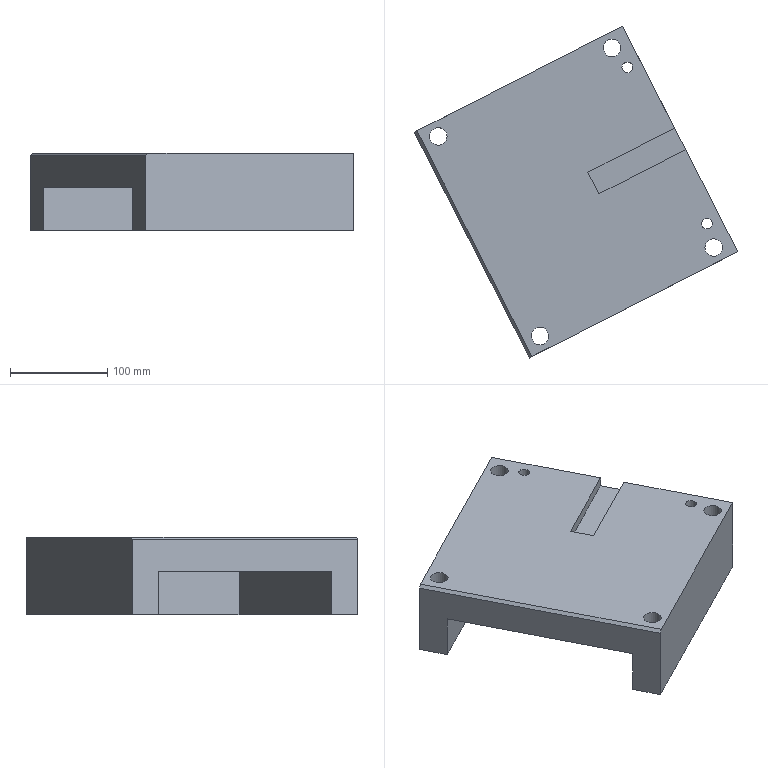Part | NX | features solid 2 | 1 solid | 29 faces | box 331.879 x 340.619 x 80 mm | volume 2957078 mm3 | plane 19 | cylinder 10 | commonest cylinder face diameters 18 x4 26 x4 11 x2
STEP:
#1=CARTESIAN_POINT('',(-1486.952,-451.806,260.));
#2=VERTEX_POINT('',#1);
#3=CARTESIAN_POINT('',(-1486.952,-451.806,250.));
#4=VERTEX_POINT('',#3);
#5=CARTESIAN_POINT('',(-1486.952,-451.806,270.));
#6=DIRECTION('',(0.,0.,-1.));
#7=VECTOR('',#6,1000.);
#8=LINE('',#5,#7);
#9=EDGE_CURVE('',#2,#4,#8,.T.);
#10=ORIENTED_EDGE('',*,*,#9,.F.);
#11=CARTESIAN_POINT('',(-1433.609,-556.499,260.));
#12=VERTEX_POINT('',#11);
#13=CARTESIAN_POINT('',(-1433.609,-556.499,260.));
#14=DIRECTION('',(-0.454,0.891,0.));
#15=VECTOR('',#14,1000.);
#16=LINE('',#13,#15);
#17=EDGE_CURVE('',#12,#2,#16,.T.);
#18=ORIENTED_EDGE('',*,*,#17,.F.);
#19=CARTESIAN_POINT('',(-1433.609,-556.499,180.));
#20=VERTEX_POINT('',#19);
#21=CARTESIAN_POINT('',(-1433.609,-556.499,260.));
#22=DIRECTION('',(0.,0.,-1.));
#23=VECTOR('',#22,1000.);
#24=LINE('',#21,#23);
#25=EDGE_CURVE('',#12,#20,#24,.T.);
#26=ORIENTED_EDGE('',*,*,#25,.T.);
#27=CARTESIAN_POINT('',(-1551.646,-324.838,180.));
#28=VERTEX_POINT('',#27);
#29=CARTESIAN_POINT('',(-1433.609,-556.499,180.));
#30=DIRECTION('',(-0.454,0.891,0.));
#31=VECTOR('',#30,1000.);
#32=LINE('',#29,#31);
#33=EDGE_CURVE('',#20,#28,#32,.T.);
#34=ORIENTED_EDGE('',*,*,#33,.T.);
#35=CARTESIAN_POINT('',(-1551.646,-324.838,260.));
#36=VERTEX_POINT('',#35);
#37=CARTESIAN_POINT('',(-1551.646,-324.838,260.));
#38=DIRECTION('',(0.,0.,-1.));
#39=VECTOR('',#38,1000.);
#40=LINE('',#37,#39);
#41=EDGE_CURVE('',#36,#28,#40,.T.);
#42=ORIENTED_EDGE('',*,*,#41,.F.);
#43=CARTESIAN_POINT('',(-1498.302,-429.531,260.));
#44=VERTEX_POINT('',#43);
#45=CARTESIAN_POINT('',(-1433.609,-556.499,260.));
#46=DIRECTION('',(-0.454,0.891,0.));
#47=VECTOR('',#46,1000.);
#48=LINE('',#45,#47);
#49=EDGE_CURVE('',#44,#36,#48,.T.);
#50=ORIENTED_EDGE('',*,*,#49,.F.);
#51=CARTESIAN_POINT('',(-1498.302,-429.531,250.));
#52=VERTEX_POINT('',#51);
#53=CARTESIAN_POINT('',(-1498.302,-429.531,250.));
#54=DIRECTION('',(0.,0.,1.));
#55=VECTOR('',#54,1000.);
#56=LINE('',#53,#55);
#57=EDGE_CURVE('',#52,#44,#56,.T.);
#58=ORIENTED_EDGE('',*,*,#57,.F.);
#59=CARTESIAN_POINT('',(-1486.952,-451.806,250.));
#60=DIRECTION('',(-0.454,0.891,0.));
#61=VECTOR('',#60,1000.);
#62=LINE('',#59,#61);
#63=EDGE_CURVE('',#4,#52,#62,.T.);
#64=ORIENTED_EDGE('',*,*,#63,.F.);
#65=EDGE_LOOP('',(#10,#18,#26,#34,#42,#50,#58,#64));
#66=FACE_BOUND('',#65,.T.);
#67=CARTESIAN_POINT('',(-1433.609,-556.499,260.));
#68=DIRECTION('',(-0.891,-0.454,0.));
#69=DIRECTION('',(0.,0.,1.));
#70=AXIS2_PLACEMENT_3D('',#67,#68,#69);
#71=PLANE('',#70);
#72=ADVANCED_FACE('',(#66),#71,.F.);
#73=CARTESIAN_POINT('',(-1628.42,-638.926,260.));
#74=VERTEX_POINT('',#73);
#75=CARTESIAN_POINT('',(-1636.44,-643.012,260.));
#76=DIRECTION('',(0.,0.,-1.));
#77=DIRECTION('',(0.891,0.454,0.));
#78=AXIS2_PLACEMENT_3D('',#75,#76,#77);
#79=CIRCLE('',#78,9.);
#80=EDGE_CURVE('',#74,#74,#79,.T.);
#81=ORIENTED_EDGE('',*,*,#80,.T.);
#82=EDGE_LOOP('',(#81));
#83=FACE_BOUND('',#82,.T.);
#84=CARTESIAN_POINT('',(-1450.219,-548.128,260.));
#85=VERTEX_POINT('',#84);
#86=CARTESIAN_POINT('',(-1458.238,-552.214,260.));
#87=DIRECTION('',(0.,0.,-1.));
#88=DIRECTION('',(0.891,0.454,0.));
#89=AXIS2_PLACEMENT_3D('',#86,#87,#88);
#90=CIRCLE('',#89,9.);
#91=EDGE_CURVE('',#85,#85,#90,.T.);
#92=ORIENTED_EDGE('',*,*,#91,.T.);
#93=EDGE_LOOP('',(#92));
#94=FACE_BOUND('',#93,.T.);
#95=CARTESIAN_POINT('',(-1460.232,-525.172,260.));
#96=VERTEX_POINT('',#95);
#97=CARTESIAN_POINT('',(-1465.133,-527.669,260.));
#98=DIRECTION('',(0.,0.,-1.));
#99=DIRECTION('',(0.891,0.454,0.));
#100=AXIS2_PLACEMENT_3D('',#97,#98,#99);
#101=CIRCLE('',#100,5.5);
#102=EDGE_CURVE('',#96,#96,#101,.T.);
#103=ORIENTED_EDGE('',*,*,#102,.T.);
#104=EDGE_LOOP('',(#103));
#105=FACE_BOUND('',#104,.T.);
#106=CARTESIAN_POINT('',(-1541.951,-364.791,260.));
#107=VERTEX_POINT('',#106);
#108=CARTESIAN_POINT('',(-1546.851,-367.288,260.));
#109=DIRECTION('',(0.,0.,-1.));
#110=DIRECTION('',(0.891,0.454,0.));
#111=AXIS2_PLACEMENT_3D('',#108,#109,#110);
#112=CIRCLE('',#111,5.5);
#113=EDGE_CURVE('',#107,#107,#112,.T.);
#114=ORIENTED_EDGE('',*,*,#113,.T.);
#115=EDGE_LOOP('',(#114));
#116=FACE_BOUND('',#115,.T.);
#117=CARTESIAN_POINT('',(-1554.637,-343.197,260.));
#118=VERTEX_POINT('',#117);
#119=CARTESIAN_POINT('',(-1562.656,-347.283,260.));
#120=DIRECTION('',(0.,0.,-1.));
#121=DIRECTION('',(0.891,0.454,0.));
#122=AXIS2_PLACEMENT_3D('',#119,#120,#121);
#123=CIRCLE('',#122,9.);
#124=EDGE_CURVE('',#118,#118,#123,.T.);
#125=ORIENTED_EDGE('',*,*,#124,.T.);
#126=EDGE_LOOP('',(#125));
#127=FACE_BOUND('',#126,.T.);
#128=CARTESIAN_POINT('',(-1732.838,-433.995,260.));
#129=VERTEX_POINT('',#128);
#130=CARTESIAN_POINT('',(-1740.857,-438.081,260.));
#131=DIRECTION('',(0.,0.,-1.));
#132=DIRECTION('',(0.891,0.454,0.));
#133=AXIS2_PLACEMENT_3D('',#130,#131,#132);
#134=CIRCLE('',#133,9.);
#135=EDGE_CURVE('',#129,#129,#134,.T.);
#136=ORIENTED_EDGE('',*,*,#135,.T.);
#137=EDGE_LOOP('',(#136));
#138=FACE_BOUND('',#137,.T.);
#139=CARTESIAN_POINT('',(-1576.053,-497.205,260.));
#140=VERTEX_POINT('',#139);
#141=CARTESIAN_POINT('',(-1587.403,-474.93,260.));
#142=VERTEX_POINT('',#141);
#143=CARTESIAN_POINT('',(-1522.709,-601.899,260.));
#144=DIRECTION('',(-0.454,0.891,0.));
#145=VECTOR('',#144,1000.);
#146=LINE('',#143,#145);
#147=EDGE_CURVE('',#140,#142,#146,.T.);
#148=ORIENTED_EDGE('',*,*,#147,.T.);
#149=CARTESIAN_POINT('',(-1498.302,-429.531,260.));
#150=DIRECTION('',(-0.891,-0.454,0.));
#151=VECTOR('',#150,1000.);
#152=LINE('',#149,#151);
#153=EDGE_CURVE('',#44,#142,#152,.T.);
#154=ORIENTED_EDGE('',*,*,#153,.F.);
#155=ORIENTED_EDGE('',*,*,#49,.T.);
#156=CARTESIAN_POINT('',(-1762.815,-432.434,260.));
#157=VERTEX_POINT('',#156);
#158=CARTESIAN_POINT('',(-1551.646,-324.838,260.));
#159=DIRECTION('',(-0.891,-0.454,0.));
#160=VECTOR('',#159,1000.);
#161=LINE('',#158,#160);
#162=EDGE_CURVE('',#36,#157,#161,.T.);
#163=ORIENTED_EDGE('',*,*,#162,.T.);
#164=CARTESIAN_POINT('',(-1644.777,-664.095,260.));
#165=VERTEX_POINT('',#164);
#166=CARTESIAN_POINT('',(-1644.777,-664.095,260.));
#167=DIRECTION('',(-0.454,0.891,0.));
#168=VECTOR('',#167,1000.);
#169=LINE('',#166,#168);
#170=EDGE_CURVE('',#165,#157,#169,.T.);
#171=ORIENTED_EDGE('',*,*,#170,.F.);
#172=CARTESIAN_POINT('',(-1433.609,-556.499,260.));
#173=DIRECTION('',(-0.891,-0.454,0.));
#174=VECTOR('',#173,1000.);
#175=LINE('',#172,#174);
#176=EDGE_CURVE('',#12,#165,#175,.T.);
#177=ORIENTED_EDGE('',*,*,#176,.F.);
#178=ORIENTED_EDGE('',*,*,#17,.T.);
#179=CARTESIAN_POINT('',(-1486.952,-451.806,260.));
#180=DIRECTION('',(0.891,0.454,0.));
#181=VECTOR('',#180,1000.);
#182=LINE('',#179,#181);
#183=EDGE_CURVE('',#140,#2,#182,.T.);
#184=ORIENTED_EDGE('',*,*,#183,.F.);
#185=EDGE_LOOP('',(#148,#154,#155,#163,#171,#177,#178,#184));
#186=FACE_BOUND('',#185,.T.);
#187=CARTESIAN_POINT('',(-1433.609,-556.499,260.));
#188=DIRECTION('',(0.,0.,1.));
#189=DIRECTION('',(0.891,0.454,0.));
#190=AXIS2_PLACEMENT_3D('',#187,#188,#189);
#191=PLANE('',#190);
#192=ADVANCED_FACE('',(#83,#94,#105,#116,#127,#138,#186),#191,.T.);
#193=CARTESIAN_POINT('',(-1647.45,-665.457,257.));
#194=VERTEX_POINT('',#193);
#195=CARTESIAN_POINT('',(-1765.488,-433.795,257.));
#196=VERTEX_POINT('',#195);
#197=CARTESIAN_POINT('',(-1647.45,-665.457,257.));
#198=DIRECTION('',(-0.454,0.891,0.));
#199=VECTOR('',#198,1000.);
#200=LINE('',#197,#199);
#201=EDGE_CURVE('',#194,#196,#200,.T.);
#202=ORIENTED_EDGE('',*,*,#201,.F.);
#203=CARTESIAN_POINT('',(-1644.777,-664.095,260.));
#204=DIRECTION('',(-0.63,-0.321,-0.7071));
#205=VECTOR('',#204,1000.);
#206=LINE('',#203,#205);
#207=EDGE_CURVE('',#165,#194,#206,.T.);
#208=ORIENTED_EDGE('',*,*,#207,.F.);
#209=ORIENTED_EDGE('',*,*,#170,.T.);
#210=CARTESIAN_POINT('',(-1762.815,-432.434,260.));
#211=DIRECTION('',(-0.63,-0.321,-0.7071));
#212=VECTOR('',#211,1000.);
#213=LINE('',#210,#212);
#214=EDGE_CURVE('',#157,#196,#213,.T.);
#215=ORIENTED_EDGE('',*,*,#214,.T.);
#216=EDGE_LOOP('',(#202,#208,#209,#215));
#217=FACE_BOUND('',#216,.T.);
#218=CARTESIAN_POINT('',(-1644.777,-664.095,260.));
#219=DIRECTION('',(-0.63,-0.321,0.7071));
#220=DIRECTION('',(0.63,0.321,0.7071));
#221=AXIS2_PLACEMENT_3D('',#218,#219,#220);
#222=PLANE('',#221);
#223=ADVANCED_FACE('',(#217),#222,.T.);
#224=CARTESIAN_POINT('',(-1661.07,-638.727,225.));
#225=VERTEX_POINT('',#224);
#226=CARTESIAN_POINT('',(-1661.07,-638.727,180.));
#227=VERTEX_POINT('',#226);
#228=CARTESIAN_POINT('',(-1661.07,-638.727,185.));
#229=DIRECTION('',(0.,0.,-1.));
#230=VECTOR('',#229,1000.);
#231=LINE('',#228,#230);
#232=EDGE_CURVE('',#225,#227,#231,.T.);
#233=ORIENTED_EDGE('',*,*,#232,.T.);
#234=CARTESIAN_POINT('',(-1647.45,-665.457,180.));
#235=VERTEX_POINT('',#234);
#236=CARTESIAN_POINT('',(-1647.45,-665.457,180.));
#237=DIRECTION('',(-0.454,0.891,0.));
#238=VECTOR('',#237,1000.);
#239=LINE('',#236,#238);
#240=EDGE_CURVE('',#227,#235,#239,.F.);
#241=ORIENTED_EDGE('',*,*,#240,.T.);
#242=CARTESIAN_POINT('',(-1647.45,-665.457,185.));
#243=DIRECTION('',(0.,0.,-1.));
#244=VECTOR('',#243,1000.);
#245=LINE('',#242,#244);
#246=EDGE_CURVE('',#194,#235,#245,.T.);
#247=ORIENTED_EDGE('',*,*,#246,.F.);
#248=ORIENTED_EDGE('',*,*,#201,.T.);
#249=CARTESIAN_POINT('',(-1765.488,-433.795,180.));
#250=VERTEX_POINT('',#249);
#251=CARTESIAN_POINT('',(-1765.488,-433.795,250.));
#252=DIRECTION('',(0.,0.,-1.));
#253=VECTOR('',#252,1000.);
#254=LINE('',#251,#253);
#255=EDGE_CURVE('',#196,#250,#254,.T.);
#256=ORIENTED_EDGE('',*,*,#255,.T.);
#257=CARTESIAN_POINT('',(-1751.868,-460.526,180.));
#258=VERTEX_POINT('',#257);
#259=CARTESIAN_POINT('',(-1765.488,-433.795,180.));
#260=DIRECTION('',(0.454,-0.891,0.));
#261=VECTOR('',#260,1000.);
#262=LINE('',#259,#261);
#263=EDGE_CURVE('',#250,#258,#262,.T.);
#264=ORIENTED_EDGE('',*,*,#263,.T.);
#265=CARTESIAN_POINT('',(-1751.868,-460.526,225.));
#266=VERTEX_POINT('',#265);
#267=CARTESIAN_POINT('',(-1751.868,-460.526,250.));
#268=DIRECTION('',(0.,0.,-1.));
#269=VECTOR('',#268,1000.);
#270=LINE('',#267,#269);
#271=EDGE_CURVE('',#266,#258,#270,.T.);
#272=ORIENTED_EDGE('',*,*,#271,.F.);
#273=CARTESIAN_POINT('',(-1661.07,-638.727,225.));
#274=DIRECTION('',(-0.454,0.891,0.));
#275=VECTOR('',#274,1000.);
#276=LINE('',#273,#275);
#277=EDGE_CURVE('',#225,#266,#276,.T.);
#278=ORIENTED_EDGE('',*,*,#277,.F.);
#279=EDGE_LOOP('',(#233,#241,#247,#248,#256,#264,#272,#278));
#280=FACE_BOUND('',#279,.T.);
#281=CARTESIAN_POINT('',(-1647.45,-665.457,185.));
#282=DIRECTION('',(-0.891,-0.454,0.));
#283=DIRECTION('',(0.,0.,1.));
#284=AXIS2_PLACEMENT_3D('',#281,#282,#283);
#285=PLANE('',#284);
#286=ADVANCED_FACE('',(#280),#285,.T.);
#287=CARTESIAN_POINT('',(-1541.951,-364.791,180.));
#288=VERTEX_POINT('',#287);
#289=CARTESIAN_POINT('',(-1546.851,-367.288,180.));
#290=DIRECTION('',(0.,0.,-1.));
#291=DIRECTION('',(0.891,0.454,0.));
#292=AXIS2_PLACEMENT_3D('',#289,#290,#291);
#293=CIRCLE('',#292,5.5);
#294=EDGE_CURVE('',#288,#288,#293,.T.);
#295=ORIENTED_EDGE('',*,*,#294,.F.);
#296=EDGE_LOOP('',(#295));
#297=FACE_BOUND('',#296,.T.);
#298=CARTESIAN_POINT('',(-1460.232,-525.172,180.));
#299=VERTEX_POINT('',#298);
#300=CARTESIAN_POINT('',(-1465.133,-527.669,180.));
#301=DIRECTION('',(0.,0.,-1.));
#302=DIRECTION('',(0.891,0.454,0.));
#303=AXIS2_PLACEMENT_3D('',#300,#301,#302);
#304=CIRCLE('',#303,5.5);
#305=EDGE_CURVE('',#299,#299,#304,.T.);
#306=ORIENTED_EDGE('',*,*,#305,.F.);
#307=EDGE_LOOP('',(#306));
#308=FACE_BOUND('',#307,.T.);
#309=CARTESIAN_POINT('',(-1729.274,-432.179,180.));
#310=VERTEX_POINT('',#309);
#311=CARTESIAN_POINT('',(-1740.857,-438.081,180.));
#312=DIRECTION('',(0.,0.,-1.));
#313=DIRECTION('',(0.891,0.454,0.));
#314=AXIS2_PLACEMENT_3D('',#311,#312,#313);
#315=CIRCLE('',#314,13.);
#316=EDGE_CURVE('',#310,#310,#315,.T.);
#317=ORIENTED_EDGE('',*,*,#316,.F.);
#318=EDGE_LOOP('',(#317));
#319=FACE_BOUND('',#318,.T.);
#320=CARTESIAN_POINT('',(-1551.073,-341.381,180.));
#321=VERTEX_POINT('',#320);
#322=CARTESIAN_POINT('',(-1562.656,-347.283,180.));
#323=DIRECTION('',(0.,0.,-1.));
#324=DIRECTION('',(0.891,0.454,0.));
#325=AXIS2_PLACEMENT_3D('',#322,#323,#324);
#326=CIRCLE('',#325,13.);
#327=EDGE_CURVE('',#321,#321,#326,.T.);
#328=ORIENTED_EDGE('',*,*,#327,.F.);
#329=EDGE_LOOP('',(#328));
#330=FACE_BOUND('',#329,.T.);
#331=CARTESIAN_POINT('',(-1624.856,-637.11,180.));
#332=VERTEX_POINT('',#331);
#333=CARTESIAN_POINT('',(-1636.44,-643.012,180.));
#334=DIRECTION('',(0.,0.,-1.));
#335=DIRECTION('',(0.891,0.454,0.));
#336=AXIS2_PLACEMENT_3D('',#333,#334,#335);
#337=CIRCLE('',#336,13.);
#338=EDGE_CURVE('',#332,#332,#337,.T.);
#339=ORIENTED_EDGE('',*,*,#338,.F.);
#340=EDGE_LOOP('',(#339));
#341=FACE_BOUND('',#340,.T.);
#342=CARTESIAN_POINT('',(-1446.655,-546.312,180.));
#343=VERTEX_POINT('',#342);
#344=CARTESIAN_POINT('',(-1458.238,-552.214,180.));
#345=DIRECTION('',(0.,0.,-1.));
#346=DIRECTION('',(0.891,0.454,0.));
#347=AXIS2_PLACEMENT_3D('',#344,#345,#346);
#348=CIRCLE('',#347,13.);
#349=EDGE_CURVE('',#343,#343,#348,.T.);
#350=ORIENTED_EDGE('',*,*,#349,.F.);
#351=EDGE_LOOP('',(#350));
#352=FACE_BOUND('',#351,.T.);
#353=ORIENTED_EDGE('',*,*,#33,.F.);
#354=CARTESIAN_POINT('',(-1433.609,-556.499,180.));
#355=DIRECTION('',(-0.891,-0.454,0.));
#356=VECTOR('',#355,1000.);
#357=LINE('',#354,#356);
#358=EDGE_CURVE('',#20,#235,#357,.T.);
#359=ORIENTED_EDGE('',*,*,#358,.T.);
#360=ORIENTED_EDGE('',*,*,#240,.F.);
#361=CARTESIAN_POINT('',(-1473.958,-543.389,180.));
#362=VERTEX_POINT('',#361);
#363=CARTESIAN_POINT('',(-1447.228,-529.769,180.));
#364=DIRECTION('',(-0.891,-0.454,0.));
#365=VECTOR('',#364,1000.);
#366=LINE('',#363,#365);
#367=EDGE_CURVE('',#362,#227,#366,.T.);
#368=ORIENTED_EDGE('',*,*,#367,.F.);
#369=CARTESIAN_POINT('',(-1564.757,-365.188,180.));
#370=VERTEX_POINT('',#369);
#371=CARTESIAN_POINT('',(-1473.958,-543.389,180.));
#372=DIRECTION('',(-0.454,0.891,0.));
#373=VECTOR('',#372,1000.);
#374=LINE('',#371,#373);
#375=EDGE_CURVE('',#362,#370,#374,.T.);
#376=ORIENTED_EDGE('',*,*,#375,.T.);
#377=CARTESIAN_POINT('',(-1538.026,-351.568,180.));
#378=DIRECTION('',(-0.891,-0.454,0.));
#379=VECTOR('',#378,1000.);
#380=LINE('',#377,#379);
#381=EDGE_CURVE('',#370,#258,#380,.T.);
#382=ORIENTED_EDGE('',*,*,#381,.T.);
#383=ORIENTED_EDGE('',*,*,#263,.F.);
#384=CARTESIAN_POINT('',(-1551.646,-324.838,180.));
#385=DIRECTION('',(-0.891,-0.454,0.));
#386=VECTOR('',#385,1000.);
#387=LINE('',#384,#386);
#388=EDGE_CURVE('',#28,#250,#387,.T.);
#389=ORIENTED_EDGE('',*,*,#388,.F.);
#390=EDGE_LOOP('',(#353,#359,#360,#368,#376,#382,#383,#389));
#391=FACE_BOUND('',#390,.T.);
#392=CARTESIAN_POINT('',(-1433.609,-556.499,180.));
#393=DIRECTION('',(0.,0.,1.));
#394=DIRECTION('',(0.891,0.454,0.));
#395=AXIS2_PLACEMENT_3D('',#392,#393,#394);
#396=PLANE('',#395);
#397=ADVANCED_FACE('',(#297,#308,#319,#330,#341,#352,#391),#396,.F.);
#398=ORIENTED_EDGE('',*,*,#207,.T.);
#399=ORIENTED_EDGE('',*,*,#246,.T.);
#400=ORIENTED_EDGE('',*,*,#358,.F.);
#401=ORIENTED_EDGE('',*,*,#25,.F.);
#402=ORIENTED_EDGE('',*,*,#176,.T.);
#403=EDGE_LOOP('',(#398,#399,#400,#401,#402));
#404=FACE_BOUND('',#403,.T.);
#405=CARTESIAN_POINT('',(-1647.45,-665.457,257.));
#406=DIRECTION('',(-0.454,0.891,0.));
#407=DIRECTION('',(0.,0.,-1.));
#408=AXIS2_PLACEMENT_3D('',#405,#406,#407);
#409=PLANE('',#408);
#410=ADVANCED_FACE('',(#404),#409,.F.);
#411=CARTESIAN_POINT('',(-1473.958,-543.389,225.));
#412=VERTEX_POINT('',#411);
#413=CARTESIAN_POINT('',(-1473.958,-543.389,225.));
#414=DIRECTION('',(0.,0.,-1.));
#415=VECTOR('',#414,1000.);
#416=LINE('',#413,#415);
#417=EDGE_CURVE('',#412,#362,#416,.T.);
#418=ORIENTED_EDGE('',*,*,#417,.T.);
#419=ORIENTED_EDGE('',*,*,#367,.T.);
#420=ORIENTED_EDGE('',*,*,#232,.F.);
#421=CARTESIAN_POINT('',(-1487.324,-550.199,225.));
#422=DIRECTION('',(0.891,0.454,0.));
#423=VECTOR('',#422,1000.);
#424=LINE('',#421,#423);
#425=EDGE_CURVE('',#225,#412,#424,.T.);
#426=ORIENTED_EDGE('',*,*,#425,.T.);
#427=EDGE_LOOP('',(#418,#419,#420,#426));
#428=FACE_BOUND('',#427,.T.);
#429=CARTESIAN_POINT('',(-1661.07,-638.727,257.));
#430=DIRECTION('',(-0.454,0.891,0.));
#431=DIRECTION('',(0.,0.,-1.));
#432=AXIS2_PLACEMENT_3D('',#429,#430,#431);
#433=PLANE('',#432);
#434=ADVANCED_FACE('',(#428),#433,.T.);
#435=CARTESIAN_POINT('',(-1564.757,-365.188,225.));
#436=VERTEX_POINT('',#435);
#437=CARTESIAN_POINT('',(-1578.122,-371.998,225.));
#438=DIRECTION('',(0.891,0.454,0.));
#439=VECTOR('',#438,1000.);
#440=LINE('',#437,#439);
#441=EDGE_CURVE('',#266,#436,#440,.T.);
#442=ORIENTED_EDGE('',*,*,#441,.T.);
#443=CARTESIAN_POINT('',(-1473.958,-543.389,225.));
#444=DIRECTION('',(-0.454,0.891,0.));
#445=VECTOR('',#444,1000.);
#446=LINE('',#443,#445);
#447=EDGE_CURVE('',#412,#436,#446,.T.);
#448=ORIENTED_EDGE('',*,*,#447,.F.);
#449=ORIENTED_EDGE('',*,*,#425,.F.);
#450=ORIENTED_EDGE('',*,*,#277,.T.);
#451=EDGE_LOOP('',(#442,#448,#449,#450));
#452=FACE_BOUND('',#451,.T.);
#453=CARTESIAN_POINT('',(-1487.324,-550.199,225.));
#454=DIRECTION('',(0.,0.,-1.));
#455=DIRECTION('',(-0.891,-0.454,0.));
#456=AXIS2_PLACEMENT_3D('',#453,#454,#455);
#457=PLANE('',#456);
#458=ADVANCED_FACE('',(#452),#457,.T.);
#459=CARTESIAN_POINT('',(-1564.757,-365.188,225.));
#460=DIRECTION('',(0.,0.,-1.));
#461=VECTOR('',#460,1000.);
#462=LINE('',#459,#461);
#463=EDGE_CURVE('',#436,#370,#462,.T.);
#464=ORIENTED_EDGE('',*,*,#463,.T.);
#465=ORIENTED_EDGE('',*,*,#375,.F.);
#466=ORIENTED_EDGE('',*,*,#417,.F.);
#467=ORIENTED_EDGE('',*,*,#447,.T.);
#468=EDGE_LOOP('',(#464,#465,#466,#467));
#469=FACE_BOUND('',#468,.T.);
#470=CARTESIAN_POINT('',(-1473.958,-543.389,225.));
#471=DIRECTION('',(-0.891,-0.454,0.));
#472=DIRECTION('',(0.,0.,1.));
#473=AXIS2_PLACEMENT_3D('',#470,#471,#472);
#474=PLANE('',#473);
#475=ADVANCED_FACE('',(#469),#474,.T.);
#476=ORIENTED_EDGE('',*,*,#255,.F.);
#477=ORIENTED_EDGE('',*,*,#214,.F.);
#478=ORIENTED_EDGE('',*,*,#162,.F.);
#479=ORIENTED_EDGE('',*,*,#41,.T.);
#480=ORIENTED_EDGE('',*,*,#388,.T.);
#481=EDGE_LOOP('',(#476,#477,#478,#479,#480));
#482=FACE_BOUND('',#481,.T.);
#483=CARTESIAN_POINT('',(-1765.488,-433.795,180.));
#484=DIRECTION('',(0.454,-0.891,0.));
#485=DIRECTION('',(0.,0.,1.));
#486=AXIS2_PLACEMENT_3D('',#483,#484,#485);
#487=PLANE('',#486);
#488=ADVANCED_FACE('',(#482),#487,.F.);
#489=ORIENTED_EDGE('',*,*,#271,.T.);
#490=ORIENTED_EDGE('',*,*,#381,.F.);
#491=ORIENTED_EDGE('',*,*,#463,.F.);
#492=ORIENTED_EDGE('',*,*,#441,.F.);
#493=EDGE_LOOP('',(#489,#490,#491,#492));
#494=FACE_BOUND('',#493,.T.);
#495=CARTESIAN_POINT('',(-1751.868,-460.526,180.));
#496=DIRECTION('',(0.454,-0.891,0.));
#497=DIRECTION('',(0.,0.,1.));
#498=AXIS2_PLACEMENT_3D('',#495,#496,#497);
#499=PLANE('',#498);
#500=ADVANCED_FACE('',(#494),#499,.T.);
#501=CARTESIAN_POINT('',(-1446.655,-546.312,200.));
#502=VERTEX_POINT('',#501);
#503=CARTESIAN_POINT('',(-1458.238,-552.214,200.));
#504=DIRECTION('',(0.,0.,-1.));
#505=DIRECTION('',(0.891,0.454,0.));
#506=AXIS2_PLACEMENT_3D('',#503,#504,#505);
#507=CIRCLE('',#506,13.);
#508=EDGE_CURVE('',#502,#502,#507,.T.);
#509=ORIENTED_EDGE('',*,*,#508,.F.);
#510=EDGE_LOOP('',(#509));
#511=FACE_BOUND('',#510,.T.);
#512=ORIENTED_EDGE('',*,*,#349,.T.);
#513=EDGE_LOOP('',(#512));
#514=FACE_BOUND('',#513,.T.);
#515=CARTESIAN_POINT('',(-1458.238,-552.214,169.));
#516=DIRECTION('',(0.,0.,1.));
#517=DIRECTION('',(0.891,0.454,0.));
#518=AXIS2_PLACEMENT_3D('',#515,#516,#517);
#519=CYLINDRICAL_SURFACE('',#518,13.);
#520=ADVANCED_FACE('',(#511,#514),#519,.F.);
#521=CARTESIAN_POINT('',(-1450.219,-548.128,200.));
#522=VERTEX_POINT('',#521);
#523=CARTESIAN_POINT('',(-1458.238,-552.214,200.));
#524=DIRECTION('',(0.,0.,-1.));
#525=DIRECTION('',(0.891,0.454,0.));
#526=AXIS2_PLACEMENT_3D('',#523,#524,#525);
#527=CIRCLE('',#526,9.);
#528=EDGE_CURVE('',#522,#522,#527,.T.);
#529=ORIENTED_EDGE('',*,*,#528,.F.);
#530=EDGE_LOOP('',(#529));
#531=FACE_BOUND('',#530,.T.);
#532=ORIENTED_EDGE('',*,*,#508,.T.);
#533=EDGE_LOOP('',(#532));
#534=FACE_BOUND('',#533,.T.);
#535=CARTESIAN_POINT('',(-1458.238,-552.214,200.));
#536=DIRECTION('',(0.,0.,1.));
#537=DIRECTION('',(0.891,0.454,0.));
#538=AXIS2_PLACEMENT_3D('',#535,#536,#537);
#539=PLANE('',#538);
#540=ADVANCED_FACE('',(#531,#534),#539,.F.);
#541=CARTESIAN_POINT('',(-1624.856,-637.11,200.));
#542=VERTEX_POINT('',#541);
#543=CARTESIAN_POINT('',(-1636.44,-643.012,200.));
#544=DIRECTION('',(0.,0.,-1.));
#545=DIRECTION('',(0.891,0.454,0.));
#546=AXIS2_PLACEMENT_3D('',#543,#544,#545);
#547=CIRCLE('',#546,13.);
#548=EDGE_CURVE('',#542,#542,#547,.T.);
#549=ORIENTED_EDGE('',*,*,#548,.F.);
#550=EDGE_LOOP('',(#549));
#551=FACE_BOUND('',#550,.T.);
#552=ORIENTED_EDGE('',*,*,#338,.T.);
#553=EDGE_LOOP('',(#552));
#554=FACE_BOUND('',#553,.T.);
#555=CARTESIAN_POINT('',(-1636.44,-643.012,169.));
#556=DIRECTION('',(0.,0.,1.));
#557=DIRECTION('',(0.891,0.454,0.));
#558=AXIS2_PLACEMENT_3D('',#555,#556,#557);
#559=CYLINDRICAL_SURFACE('',#558,13.);
#560=ADVANCED_FACE('',(#551,#554),#559,.F.);
#561=CARTESIAN_POINT('',(-1628.42,-638.926,200.));
#562=VERTEX_POINT('',#561);
#563=CARTESIAN_POINT('',(-1636.44,-643.012,200.));
#564=DIRECTION('',(0.,0.,-1.));
#565=DIRECTION('',(0.891,0.454,0.));
#566=AXIS2_PLACEMENT_3D('',#563,#564,#565);
#567=CIRCLE('',#566,9.);
#568=EDGE_CURVE('',#562,#562,#567,.T.);
#569=ORIENTED_EDGE('',*,*,#568,.F.);
#570=EDGE_LOOP('',(#569));
#571=FACE_BOUND('',#570,.T.);
#572=ORIENTED_EDGE('',*,*,#548,.T.);
#573=EDGE_LOOP('',(#572));
#574=FACE_BOUND('',#573,.T.);
#575=CARTESIAN_POINT('',(-1636.44,-643.012,200.));
#576=DIRECTION('',(0.,0.,1.));
#577=DIRECTION('',(0.891,0.454,0.));
#578=AXIS2_PLACEMENT_3D('',#575,#576,#577);
#579=PLANE('',#578);
#580=ADVANCED_FACE('',(#571,#574),#579,.F.);
#581=CARTESIAN_POINT('',(-1551.073,-341.381,200.));
#582=VERTEX_POINT('',#581);
#583=CARTESIAN_POINT('',(-1562.656,-347.283,200.));
#584=DIRECTION('',(0.,0.,-1.));
#585=DIRECTION('',(0.891,0.454,0.));
#586=AXIS2_PLACEMENT_3D('',#583,#584,#585);
#587=CIRCLE('',#586,13.);
#588=EDGE_CURVE('',#582,#582,#587,.T.);
#589=ORIENTED_EDGE('',*,*,#588,.F.);
#590=EDGE_LOOP('',(#589));
#591=FACE_BOUND('',#590,.T.);
#592=ORIENTED_EDGE('',*,*,#327,.T.);
#593=EDGE_LOOP('',(#592));
#594=FACE_BOUND('',#593,.T.);
#595=CARTESIAN_POINT('',(-1562.656,-347.283,169.));
#596=DIRECTION('',(0.,0.,1.));
#597=DIRECTION('',(0.891,0.454,0.));
#598=AXIS2_PLACEMENT_3D('',#595,#596,#597);
#599=CYLINDRICAL_SURFACE('',#598,13.);
#600=ADVANCED_FACE('',(#591,#594),#599,.F.);
#601=CARTESIAN_POINT('',(-1554.637,-343.197,200.));
#602=VERTEX_POINT('',#601);
#603=CARTESIAN_POINT('',(-1562.656,-347.283,200.));
#604=DIRECTION('',(0.,0.,-1.));
#605=DIRECTION('',(0.891,0.454,0.));
#606=AXIS2_PLACEMENT_3D('',#603,#604,#605);
#607=CIRCLE('',#606,9.);
#608=EDGE_CURVE('',#602,#602,#607,.T.);
#609=ORIENTED_EDGE('',*,*,#608,.F.);
#610=EDGE_LOOP('',(#609));
#611=FACE_BOUND('',#610,.T.);
#612=ORIENTED_EDGE('',*,*,#588,.T.);
#613=EDGE_LOOP('',(#612));
#614=FACE_BOUND('',#613,.T.);
#615=CARTESIAN_POINT('',(-1562.656,-347.283,200.));
#616=DIRECTION('',(0.,0.,1.));
#617=DIRECTION('',(0.891,0.454,0.));
#618=AXIS2_PLACEMENT_3D('',#615,#616,#617);
#619=PLANE('',#618);
#620=ADVANCED_FACE('',(#611,#614),#619,.F.);
#621=CARTESIAN_POINT('',(-1729.274,-432.179,200.));
#622=VERTEX_POINT('',#621);
#623=CARTESIAN_POINT('',(-1740.857,-438.081,200.));
#624=DIRECTION('',(0.,0.,-1.));
#625=DIRECTION('',(0.891,0.454,0.));
#626=AXIS2_PLACEMENT_3D('',#623,#624,#625);
#627=CIRCLE('',#626,13.);
#628=EDGE_CURVE('',#622,#622,#627,.T.);
#629=ORIENTED_EDGE('',*,*,#628,.F.);
#630=EDGE_LOOP('',(#629));
#631=FACE_BOUND('',#630,.T.);
#632=ORIENTED_EDGE('',*,*,#316,.T.);
#633=EDGE_LOOP('',(#632));
#634=FACE_BOUND('',#633,.T.);
#635=CARTESIAN_POINT('',(-1740.857,-438.081,169.));
#636=DIRECTION('',(0.,0.,1.));
#637=DIRECTION('',(0.891,0.454,0.));
#638=AXIS2_PLACEMENT_3D('',#635,#636,#637);
#639=CYLINDRICAL_SURFACE('',#638,13.);
#640=ADVANCED_FACE('',(#631,#634),#639,.F.);
#641=CARTESIAN_POINT('',(-1732.838,-433.995,200.));
#642=VERTEX_POINT('',#641);
#643=CARTESIAN_POINT('',(-1740.857,-438.081,200.));
#644=DIRECTION('',(0.,0.,-1.));
#645=DIRECTION('',(0.891,0.454,0.));
#646=AXIS2_PLACEMENT_3D('',#643,#644,#645);
#647=CIRCLE('',#646,9.);
#648=EDGE_CURVE('',#642,#642,#647,.T.);
#649=ORIENTED_EDGE('',*,*,#648,.F.);
#650=EDGE_LOOP('',(#649));
#651=FACE_BOUND('',#650,.T.);
#652=ORIENTED_EDGE('',*,*,#628,.T.);
#653=EDGE_LOOP('',(#652));
#654=FACE_BOUND('',#653,.T.);
#655=CARTESIAN_POINT('',(-1740.857,-438.081,200.));
#656=DIRECTION('',(0.,0.,1.));
#657=DIRECTION('',(0.891,0.454,0.));
#658=AXIS2_PLACEMENT_3D('',#655,#656,#657);
#659=PLANE('',#658);
#660=ADVANCED_FACE('',(#651,#654),#659,.F.);
#661=ORIENTED_EDGE('',*,*,#80,.F.);
#662=EDGE_LOOP('',(#661));
#663=FACE_BOUND('',#662,.T.);
#664=ORIENTED_EDGE('',*,*,#568,.T.);
#665=EDGE_LOOP('',(#664));
#666=FACE_BOUND('',#665,.T.);
#667=CARTESIAN_POINT('',(-1636.44,-643.012,169.));
#668=DIRECTION('',(0.,0.,1.));
#669=DIRECTION('',(0.891,0.454,0.));
#670=AXIS2_PLACEMENT_3D('',#667,#668,#669);
#671=CYLINDRICAL_SURFACE('',#670,9.);
#672=ADVANCED_FACE('',(#663,#666),#671,.F.);
#673=ORIENTED_EDGE('',*,*,#91,.F.);
#674=EDGE_LOOP('',(#673));
#675=FACE_BOUND('',#674,.T.);
#676=ORIENTED_EDGE('',*,*,#528,.T.);
#677=EDGE_LOOP('',(#676));
#678=FACE_BOUND('',#677,.T.);
#679=CARTESIAN_POINT('',(-1458.238,-552.214,169.));
#680=DIRECTION('',(0.,0.,1.));
#681=DIRECTION('',(0.891,0.454,0.));
#682=AXIS2_PLACEMENT_3D('',#679,#680,#681);
#683=CYLINDRICAL_SURFACE('',#682,9.);
#684=ADVANCED_FACE('',(#675,#678),#683,.F.);
#685=ORIENTED_EDGE('',*,*,#102,.F.);
#686=EDGE_LOOP('',(#685));
#687=FACE_BOUND('',#686,.T.);
#688=ORIENTED_EDGE('',*,*,#305,.T.);
#689=EDGE_LOOP('',(#688));
#690=FACE_BOUND('',#689,.T.);
#691=CARTESIAN_POINT('',(-1465.133,-527.669,169.));
#692=DIRECTION('',(0.,0.,1.));
#693=DIRECTION('',(0.891,0.454,0.));
#694=AXIS2_PLACEMENT_3D('',#691,#692,#693);
#695=CYLINDRICAL_SURFACE('',#694,5.5);
#696=ADVANCED_FACE('',(#687,#690),#695,.F.);
#697=ORIENTED_EDGE('',*,*,#113,.F.);
#698=EDGE_LOOP('',(#697));
#699=FACE_BOUND('',#698,.T.);
#700=ORIENTED_EDGE('',*,*,#294,.T.);
#701=EDGE_LOOP('',(#700));
#702=FACE_BOUND('',#701,.T.);
#703=CARTESIAN_POINT('',(-1546.851,-367.288,169.));
#704=DIRECTION('',(0.,0.,1.));
#705=DIRECTION('',(0.891,0.454,0.));
#706=AXIS2_PLACEMENT_3D('',#703,#704,#705);
#707=CYLINDRICAL_SURFACE('',#706,5.5);
#708=ADVANCED_FACE('',(#699,#702),#707,.F.);
#709=ORIENTED_EDGE('',*,*,#124,.F.);
#710=EDGE_LOOP('',(#709));
#711=FACE_BOUND('',#710,.T.);
#712=ORIENTED_EDGE('',*,*,#608,.T.);
#713=EDGE_LOOP('',(#712));
#714=FACE_BOUND('',#713,.T.);
#715=CARTESIAN_POINT('',(-1562.656,-347.283,169.));
#716=DIRECTION('',(0.,0.,1.));
#717=DIRECTION('',(0.891,0.454,0.));
#718=AXIS2_PLACEMENT_3D('',#715,#716,#717);
#719=CYLINDRICAL_SURFACE('',#718,9.);
#720=ADVANCED_FACE('',(#711,#714),#719,.F.);
#721=ORIENTED_EDGE('',*,*,#135,.F.);
#722=EDGE_LOOP('',(#721));
#723=FACE_BOUND('',#722,.T.);
#724=ORIENTED_EDGE('',*,*,#648,.T.);
#725=EDGE_LOOP('',(#724));
#726=FACE_BOUND('',#725,.T.);
#727=CARTESIAN_POINT('',(-1740.857,-438.081,169.));
#728=DIRECTION('',(0.,0.,1.));
#729=DIRECTION('',(0.891,0.454,0.));
#730=AXIS2_PLACEMENT_3D('',#727,#728,#729);
#731=CYLINDRICAL_SURFACE('',#730,9.);
#732=ADVANCED_FACE('',(#723,#726),#731,.F.);
#733=CARTESIAN_POINT('',(-1576.053,-497.205,250.));
#734=VERTEX_POINT('',#733);
#735=CARTESIAN_POINT('',(-1576.053,-497.205,270.));
#736=DIRECTION('',(0.,0.,-1.));
#737=VECTOR('',#736,1000.);
#738=LINE('',#735,#737);
#739=EDGE_CURVE('',#140,#734,#738,.T.);
#740=ORIENTED_EDGE('',*,*,#739,.F.);
#741=ORIENTED_EDGE('',*,*,#183,.T.);
#742=ORIENTED_EDGE('',*,*,#9,.T.);
#743=CARTESIAN_POINT('',(-1576.053,-497.205,250.));
#744=DIRECTION('',(0.891,0.454,0.));
#745=VECTOR('',#744,1000.);
#746=LINE('',#743,#745);
#747=EDGE_CURVE('',#734,#4,#746,.T.);
#748=ORIENTED_EDGE('',*,*,#747,.F.);
#749=EDGE_LOOP('',(#740,#741,#742,#748));
#750=FACE_BOUND('',#749,.T.);
#751=CARTESIAN_POINT('',(-1576.053,-497.205,270.));
#752=DIRECTION('',(-0.454,0.891,0.));
#753=DIRECTION('',(0.,0.,-1.));
#754=AXIS2_PLACEMENT_3D('',#751,#752,#753);
#755=PLANE('',#754);
#756=ADVANCED_FACE('',(#750),#755,.T.);
#757=ORIENTED_EDGE('',*,*,#63,.T.);
#758=CARTESIAN_POINT('',(-1587.403,-474.93,250.));
#759=VERTEX_POINT('',#758);
#760=CARTESIAN_POINT('',(-1587.403,-474.93,250.));
#761=DIRECTION('',(0.891,0.454,0.));
#762=VECTOR('',#761,1000.);
#763=LINE('',#760,#762);
#764=EDGE_CURVE('',#759,#52,#763,.T.);
#765=ORIENTED_EDGE('',*,*,#764,.F.);
#766=CARTESIAN_POINT('',(-1576.053,-497.205,250.));
#767=DIRECTION('',(-0.454,0.891,0.));
#768=VECTOR('',#767,1000.);
#769=LINE('',#766,#768);
#770=EDGE_CURVE('',#734,#759,#769,.T.);
#771=ORIENTED_EDGE('',*,*,#770,.F.);
#772=ORIENTED_EDGE('',*,*,#747,.T.);
#773=EDGE_LOOP('',(#757,#765,#771,#772));
#774=FACE_BOUND('',#773,.T.);
#775=CARTESIAN_POINT('',(-1576.053,-497.205,250.));
#776=DIRECTION('',(0.,0.,1.));
#777=DIRECTION('',(0.891,0.454,0.));
#778=AXIS2_PLACEMENT_3D('',#775,#776,#777);
#779=PLANE('',#778);
#780=ADVANCED_FACE('',(#774),#779,.T.);
#781=ORIENTED_EDGE('',*,*,#57,.T.);
#782=ORIENTED_EDGE('',*,*,#153,.T.);
#783=CARTESIAN_POINT('',(-1587.403,-474.93,250.));
#784=DIRECTION('',(0.,0.,1.));
#785=VECTOR('',#784,1000.);
#786=LINE('',#783,#785);
#787=EDGE_CURVE('',#759,#142,#786,.T.);
#788=ORIENTED_EDGE('',*,*,#787,.F.);
#789=ORIENTED_EDGE('',*,*,#764,.T.);
#790=EDGE_LOOP('',(#781,#782,#788,#789));
#791=FACE_BOUND('',#790,.T.);
#792=CARTESIAN_POINT('',(-1587.403,-474.93,250.));
#793=DIRECTION('',(0.454,-0.891,0.));
#794=DIRECTION('',(0.,0.,1.));
#795=AXIS2_PLACEMENT_3D('',#792,#793,#794);
#796=PLANE('',#795);
#797=ADVANCED_FACE('',(#791),#796,.T.);
#798=ORIENTED_EDGE('',*,*,#147,.F.);
#799=ORIENTED_EDGE('',*,*,#739,.T.);
#800=ORIENTED_EDGE('',*,*,#770,.T.);
#801=ORIENTED_EDGE('',*,*,#787,.T.);
#802=EDGE_LOOP('',(#798,#799,#800,#801));
#803=FACE_BOUND('',#802,.T.);
#804=CARTESIAN_POINT('',(-1576.053,-497.205,270.));
#805=DIRECTION('',(-0.891,-0.454,0.));
#806=DIRECTION('',(0.,0.,1.));
#807=AXIS2_PLACEMENT_3D('',#804,#805,#806);
#808=PLANE('',#807);
#809=ADVANCED_FACE('',(#803),#808,.F.);
#810=CLOSED_SHELL('',(#72,#192,#223,#286,#397,#410,#434,#458,#475,#488,#500,#520,#540,#560,#580,#600,#620,#640,#660,#672,#684,#696,#708,#720,#732,#756,#780,#797,#809));
#811=MANIFOLD_SOLID_BREP('',#810);
#812=(LENGTH_UNIT()NAMED_UNIT(*)SI_UNIT(.MILLI.,.METRE.));
#813=UNCERTAINTY_MEASURE_WITH_UNIT(LENGTH_MEASURE(0.00001),#812,'','');
#814=(NAMED_UNIT(*)PLANE_ANGLE_UNIT()SI_UNIT($,.RADIAN.));
#815=(NAMED_UNIT(*)SI_UNIT($,.STERADIAN.)SOLID_ANGLE_UNIT());
#816=(GEOMETRIC_REPRESENTATION_CONTEXT(3)GLOBAL_UNCERTAINTY_ASSIGNED_CONTEXT((#813))GLOBAL_UNIT_ASSIGNED_CONTEXT((#812,#814,#815))REPRESENTATION_CONTEXT('',''));
#817=ADVANCED_BREP_SHAPE_REPRESENTATION('',(#811),#816);